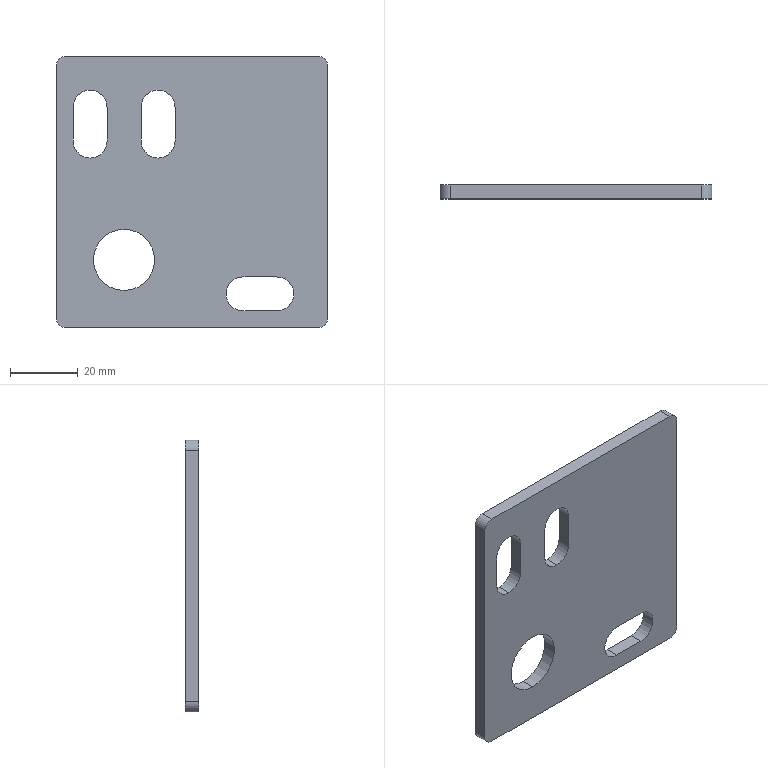Part | SolidWorks | features Extrusion 1, Fillet 1 | 1 solid | 26 faces | box 80 x 4 x 80 mm | volume 22409 mm3 | cylinder 14 | plane 12 | commonest cylinder face diameters 10 x8 6 x4 18 x2
STEP:
#1=CARTESIAN_POINT('',(-45.,4.,55.));
#2=VERTEX_POINT('',#1);
#3=CARTESIAN_POINT('',(-50.,4.,50.));
#4=VERTEX_POINT('',#3);
#5=CARTESIAN_POINT('',(-50.,4.,55.));
#6=DIRECTION('',(0.,1.,0.));
#7=DIRECTION('',(0.,0.,1.));
#8=AXIS2_PLACEMENT_3D('',#5,#6,#7);
#9=CIRCLE('',#8,5.);
#10=EDGE_CURVE('',#2,#4,#9,.T.);
#11=ORIENTED_EDGE('',*,*,#10,.T.);
#12=CARTESIAN_POINT('',(-50.,0.,50.));
#13=VERTEX_POINT('',#12);
#14=CARTESIAN_POINT('',(-50.,4.,50.));
#15=DIRECTION('',(0.,-1.,0.));
#16=VECTOR('',#15,1000.);
#17=LINE('',#14,#16);
#18=EDGE_CURVE('',#4,#13,#17,.T.);
#19=ORIENTED_EDGE('',*,*,#18,.T.);
#20=CARTESIAN_POINT('',(-45.,0.,55.));
#21=VERTEX_POINT('',#20);
#22=CARTESIAN_POINT('',(-50.,0.,55.));
#23=DIRECTION('',(0.,1.,0.));
#24=DIRECTION('',(0.,0.,1.));
#25=AXIS2_PLACEMENT_3D('',#22,#23,#24);
#26=CIRCLE('',#25,5.);
#27=EDGE_CURVE('',#21,#13,#26,.T.);
#28=ORIENTED_EDGE('',*,*,#27,.F.);
#29=CARTESIAN_POINT('',(-45.,4.,55.));
#30=DIRECTION('',(0.,-1.,0.));
#31=VECTOR('',#30,1000.);
#32=LINE('',#29,#31);
#33=EDGE_CURVE('',#2,#21,#32,.T.);
#34=ORIENTED_EDGE('',*,*,#33,.F.);
#35=EDGE_LOOP('',(#11,#19,#28,#34));
#36=FACE_OUTER_BOUND('',#35,.T.);
#37=CARTESIAN_POINT('',(-50.,4.,55.));
#38=DIRECTION('',(0.,-1.,0.));
#39=DIRECTION('',(0.,0.,-1.));
#40=AXIS2_PLACEMENT_3D('',#37,#38,#39);
#41=CYLINDRICAL_SURFACE('',#40,5.);
#42=ADVANCED_FACE('',(#36),#41,.F.);
#43=CARTESIAN_POINT('',(-65.,4.,55.));
#44=VERTEX_POINT('',#43);
#45=CARTESIAN_POINT('',(-70.,4.,50.));
#46=VERTEX_POINT('',#45);
#47=CARTESIAN_POINT('',(-70.,4.,55.));
#48=DIRECTION('',(0.,1.,0.));
#49=DIRECTION('',(0.,0.,1.));
#50=AXIS2_PLACEMENT_3D('',#47,#48,#49);
#51=CIRCLE('',#50,5.);
#52=EDGE_CURVE('',#44,#46,#51,.T.);
#53=ORIENTED_EDGE('',*,*,#52,.T.);
#54=CARTESIAN_POINT('',(-70.,0.,50.));
#55=VERTEX_POINT('',#54);
#56=CARTESIAN_POINT('',(-70.,4.,50.));
#57=DIRECTION('',(0.,-1.,0.));
#58=VECTOR('',#57,1000.);
#59=LINE('',#56,#58);
#60=EDGE_CURVE('',#46,#55,#59,.T.);
#61=ORIENTED_EDGE('',*,*,#60,.T.);
#62=CARTESIAN_POINT('',(-65.,0.,55.));
#63=VERTEX_POINT('',#62);
#64=CARTESIAN_POINT('',(-70.,0.,55.));
#65=DIRECTION('',(0.,1.,0.));
#66=DIRECTION('',(0.,0.,1.));
#67=AXIS2_PLACEMENT_3D('',#64,#65,#66);
#68=CIRCLE('',#67,5.);
#69=EDGE_CURVE('',#63,#55,#68,.T.);
#70=ORIENTED_EDGE('',*,*,#69,.F.);
#71=CARTESIAN_POINT('',(-65.,4.,55.));
#72=DIRECTION('',(0.,-1.,0.));
#73=VECTOR('',#72,1000.);
#74=LINE('',#71,#73);
#75=EDGE_CURVE('',#44,#63,#74,.T.);
#76=ORIENTED_EDGE('',*,*,#75,.F.);
#77=EDGE_LOOP('',(#53,#61,#70,#76));
#78=FACE_OUTER_BOUND('',#77,.T.);
#79=CARTESIAN_POINT('',(-70.,4.,55.));
#80=DIRECTION('',(0.,-1.,0.));
#81=DIRECTION('',(0.,0.,-1.));
#82=AXIS2_PLACEMENT_3D('',#79,#80,#81);
#83=CYLINDRICAL_SURFACE('',#82,5.);
#84=ADVANCED_FACE('',(#78),#83,.F.);
#85=CARTESIAN_POINT('',(-60.,4.,11.));
#86=VERTEX_POINT('',#85);
#87=CARTESIAN_POINT('',(-60.,4.,29.));
#88=VERTEX_POINT('',#87);
#89=CARTESIAN_POINT('',(-60.,4.,20.));
#90=DIRECTION('',(0.,1.,0.));
#91=DIRECTION('',(0.,0.,1.));
#92=AXIS2_PLACEMENT_3D('',#89,#90,#91);
#93=CIRCLE('',#92,9.);
#94=EDGE_CURVE('',#86,#88,#93,.T.);
#95=ORIENTED_EDGE('',*,*,#94,.T.);
#96=CARTESIAN_POINT('',(-60.,0.,29.));
#97=VERTEX_POINT('',#96);
#98=CARTESIAN_POINT('',(-60.,4.,29.));
#99=DIRECTION('',(0.,-1.,0.));
#100=VECTOR('',#99,1000.);
#101=LINE('',#98,#100);
#102=EDGE_CURVE('',#88,#97,#101,.T.);
#103=ORIENTED_EDGE('',*,*,#102,.T.);
#104=CARTESIAN_POINT('',(-60.,0.,11.));
#105=VERTEX_POINT('',#104);
#106=CARTESIAN_POINT('',(-60.,0.,20.));
#107=DIRECTION('',(0.,1.,0.));
#108=DIRECTION('',(0.,0.,1.));
#109=AXIS2_PLACEMENT_3D('',#106,#107,#108);
#110=CIRCLE('',#109,9.);
#111=EDGE_CURVE('',#105,#97,#110,.T.);
#112=ORIENTED_EDGE('',*,*,#111,.F.);
#113=CARTESIAN_POINT('',(-60.,4.,11.));
#114=DIRECTION('',(0.,-1.,0.));
#115=VECTOR('',#114,1000.);
#116=LINE('',#113,#115);
#117=EDGE_CURVE('',#86,#105,#116,.T.);
#118=ORIENTED_EDGE('',*,*,#117,.F.);
#119=EDGE_LOOP('',(#95,#103,#112,#118));
#120=FACE_OUTER_BOUND('',#119,.T.);
#121=CARTESIAN_POINT('',(-60.,4.,20.));
#122=DIRECTION('',(0.,-1.,0.));
#123=DIRECTION('',(0.,0.,-1.));
#124=AXIS2_PLACEMENT_3D('',#121,#122,#123);
#125=CYLINDRICAL_SURFACE('',#124,9.);
#126=ADVANCED_FACE('',(#120),#125,.F.);
#127=CARTESIAN_POINT('',(-77.,4.,80.));
#128=VERTEX_POINT('',#127);
#129=CARTESIAN_POINT('',(-3.,4.,80.));
#130=VERTEX_POINT('',#129);
#131=CARTESIAN_POINT('',(-80.,4.,80.));
#132=DIRECTION('',(1.,0.,0.));
#133=VECTOR('',#132,1000.);
#134=LINE('',#131,#133);
#135=EDGE_CURVE('',#128,#130,#134,.T.);
#136=ORIENTED_EDGE('',*,*,#135,.T.);
#137=CARTESIAN_POINT('',(0.,4.,77.));
#138=VERTEX_POINT('',#137);
#139=CARTESIAN_POINT('',(-3.,4.,77.));
#140=DIRECTION('',(0.,1.,0.));
#141=DIRECTION('',(0.,0.,1.));
#142=AXIS2_PLACEMENT_3D('',#139,#140,#141);
#143=CIRCLE('',#142,3.);
#144=EDGE_CURVE('',#130,#138,#143,.T.);
#145=ORIENTED_EDGE('',*,*,#144,.T.);
#146=CARTESIAN_POINT('',(0.,4.,3.));
#147=VERTEX_POINT('',#146);
#148=CARTESIAN_POINT('',(0.,4.,80.));
#149=DIRECTION('',(0.,0.,-1.));
#150=VECTOR('',#149,1000.);
#151=LINE('',#148,#150);
#152=EDGE_CURVE('',#138,#147,#151,.T.);
#153=ORIENTED_EDGE('',*,*,#152,.T.);
#154=CARTESIAN_POINT('',(-3.,4.,0.));
#155=VERTEX_POINT('',#154);
#156=CARTESIAN_POINT('',(-3.,4.,3.));
#157=DIRECTION('',(0.,1.,0.));
#158=DIRECTION('',(0.,0.,1.));
#159=AXIS2_PLACEMENT_3D('',#156,#157,#158);
#160=CIRCLE('',#159,3.);
#161=EDGE_CURVE('',#147,#155,#160,.T.);
#162=ORIENTED_EDGE('',*,*,#161,.T.);
#163=CARTESIAN_POINT('',(-77.,4.,0.));
#164=VERTEX_POINT('',#163);
#165=CARTESIAN_POINT('',(0.,4.,0.));
#166=DIRECTION('',(-1.,0.,0.));
#167=VECTOR('',#166,1000.);
#168=LINE('',#165,#167);
#169=EDGE_CURVE('',#155,#164,#168,.T.);
#170=ORIENTED_EDGE('',*,*,#169,.T.);
#171=CARTESIAN_POINT('',(-80.,4.,3.));
#172=VERTEX_POINT('',#171);
#173=CARTESIAN_POINT('',(-77.,4.,3.));
#174=DIRECTION('',(0.,1.,0.));
#175=DIRECTION('',(0.,0.,1.));
#176=AXIS2_PLACEMENT_3D('',#173,#174,#175);
#177=CIRCLE('',#176,3.);
#178=EDGE_CURVE('',#164,#172,#177,.T.);
#179=ORIENTED_EDGE('',*,*,#178,.T.);
#180=CARTESIAN_POINT('',(-80.,4.,77.));
#181=VERTEX_POINT('',#180);
#182=CARTESIAN_POINT('',(-80.,4.,0.));
#183=DIRECTION('',(0.,0.,1.));
#184=VECTOR('',#183,1000.);
#185=LINE('',#182,#184);
#186=EDGE_CURVE('',#172,#181,#185,.T.);
#187=ORIENTED_EDGE('',*,*,#186,.T.);
#188=CARTESIAN_POINT('',(-77.,4.,77.));
#189=DIRECTION('',(0.,1.,0.));
#190=DIRECTION('',(0.,0.,1.));
#191=AXIS2_PLACEMENT_3D('',#188,#189,#190);
#192=CIRCLE('',#191,3.);
#193=EDGE_CURVE('',#181,#128,#192,.T.);
#194=ORIENTED_EDGE('',*,*,#193,.T.);
#195=EDGE_LOOP('',(#136,#145,#153,#162,#170,#179,#187,#194));
#196=FACE_OUTER_BOUND('',#195,.T.);
#197=ORIENTED_EDGE('',*,*,#94,.F.);
#198=CARTESIAN_POINT('',(-60.,4.,20.));
#199=DIRECTION('',(0.,1.,0.));
#200=DIRECTION('',(0.,0.,1.));
#201=AXIS2_PLACEMENT_3D('',#198,#199,#200);
#202=CIRCLE('',#201,9.);
#203=EDGE_CURVE('',#88,#86,#202,.T.);
#204=ORIENTED_EDGE('',*,*,#203,.F.);
#205=EDGE_LOOP('',(#197,#204));
#206=FACE_BOUND('',#205,.T.);
#207=CARTESIAN_POINT('',(-25.,4.,15.));
#208=VERTEX_POINT('',#207);
#209=CARTESIAN_POINT('',(-15.,4.,15.));
#210=VERTEX_POINT('',#209);
#211=CARTESIAN_POINT('',(-25.,4.,15.));
#212=DIRECTION('',(1.,0.,0.));
#213=VECTOR('',#212,1000.);
#214=LINE('',#211,#213);
#215=EDGE_CURVE('',#208,#210,#214,.T.);
#216=ORIENTED_EDGE('',*,*,#215,.F.);
#217=CARTESIAN_POINT('',(-25.,4.,5.));
#218=VERTEX_POINT('',#217);
#219=CARTESIAN_POINT('',(-25.,4.,10.));
#220=DIRECTION('',(0.,1.,0.));
#221=DIRECTION('',(0.,0.,1.));
#222=AXIS2_PLACEMENT_3D('',#219,#220,#221);
#223=CIRCLE('',#222,5.);
#224=EDGE_CURVE('',#218,#208,#223,.T.);
#225=ORIENTED_EDGE('',*,*,#224,.F.);
#226=CARTESIAN_POINT('',(-15.,4.,5.));
#227=VERTEX_POINT('',#226);
#228=CARTESIAN_POINT('',(-25.,4.,5.));
#229=DIRECTION('',(-1.,0.,0.));
#230=VECTOR('',#229,1000.);
#231=LINE('',#228,#230);
#232=EDGE_CURVE('',#227,#218,#231,.T.);
#233=ORIENTED_EDGE('',*,*,#232,.F.);
#234=CARTESIAN_POINT('',(-15.,4.,10.));
#235=DIRECTION('',(0.,1.,0.));
#236=DIRECTION('',(0.,0.,1.));
#237=AXIS2_PLACEMENT_3D('',#234,#235,#236);
#238=CIRCLE('',#237,5.);
#239=EDGE_CURVE('',#210,#227,#238,.T.);
#240=ORIENTED_EDGE('',*,*,#239,.F.);
#241=EDGE_LOOP('',(#216,#225,#233,#240));
#242=FACE_BOUND('',#241,.T.);
#243=CARTESIAN_POINT('',(-75.,4.,55.));
#244=VERTEX_POINT('',#243);
#245=CARTESIAN_POINT('',(-75.,4.,65.));
#246=VERTEX_POINT('',#245);
#247=CARTESIAN_POINT('',(-75.,4.,55.));
#248=DIRECTION('',(0.,0.,1.));
#249=VECTOR('',#248,1000.);
#250=LINE('',#247,#249);
#251=EDGE_CURVE('',#244,#246,#250,.T.);
#252=ORIENTED_EDGE('',*,*,#251,.F.);
#253=CARTESIAN_POINT('',(-70.,4.,55.));
#254=DIRECTION('',(0.,1.,0.));
#255=DIRECTION('',(0.,0.,1.));
#256=AXIS2_PLACEMENT_3D('',#253,#254,#255);
#257=CIRCLE('',#256,5.);
#258=EDGE_CURVE('',#46,#244,#257,.T.);
#259=ORIENTED_EDGE('',*,*,#258,.F.);
#260=ORIENTED_EDGE('',*,*,#52,.F.);
#261=CARTESIAN_POINT('',(-65.,4.,65.));
#262=VERTEX_POINT('',#261);
#263=CARTESIAN_POINT('',(-65.,4.,55.));
#264=DIRECTION('',(0.,0.,-1.));
#265=VECTOR('',#264,1000.);
#266=LINE('',#263,#265);
#267=EDGE_CURVE('',#262,#44,#266,.T.);
#268=ORIENTED_EDGE('',*,*,#267,.F.);
#269=CARTESIAN_POINT('',(-70.,4.,65.));
#270=DIRECTION('',(0.,1.,0.));
#271=DIRECTION('',(0.,0.,1.));
#272=AXIS2_PLACEMENT_3D('',#269,#270,#271);
#273=CIRCLE('',#272,5.);
#274=EDGE_CURVE('',#246,#262,#273,.T.);
#275=ORIENTED_EDGE('',*,*,#274,.F.);
#276=EDGE_LOOP('',(#252,#259,#260,#268,#275));
#277=FACE_BOUND('',#276,.T.);
#278=CARTESIAN_POINT('',(-55.,4.,55.));
#279=VERTEX_POINT('',#278);
#280=CARTESIAN_POINT('',(-55.,4.,65.));
#281=VERTEX_POINT('',#280);
#282=CARTESIAN_POINT('',(-55.,4.,55.));
#283=DIRECTION('',(0.,0.,1.));
#284=VECTOR('',#283,1000.);
#285=LINE('',#282,#284);
#286=EDGE_CURVE('',#279,#281,#285,.T.);
#287=ORIENTED_EDGE('',*,*,#286,.F.);
#288=CARTESIAN_POINT('',(-50.,4.,55.));
#289=DIRECTION('',(0.,1.,0.));
#290=DIRECTION('',(0.,0.,1.));
#291=AXIS2_PLACEMENT_3D('',#288,#289,#290);
#292=CIRCLE('',#291,5.);
#293=EDGE_CURVE('',#4,#279,#292,.T.);
#294=ORIENTED_EDGE('',*,*,#293,.F.);
#295=ORIENTED_EDGE('',*,*,#10,.F.);
#296=CARTESIAN_POINT('',(-45.,4.,65.));
#297=VERTEX_POINT('',#296);
#298=CARTESIAN_POINT('',(-45.,4.,55.));
#299=DIRECTION('',(0.,0.,-1.));
#300=VECTOR('',#299,1000.);
#301=LINE('',#298,#300);
#302=EDGE_CURVE('',#297,#2,#301,.T.);
#303=ORIENTED_EDGE('',*,*,#302,.F.);
#304=CARTESIAN_POINT('',(-50.,4.,65.));
#305=DIRECTION('',(0.,1.,0.));
#306=DIRECTION('',(0.,0.,1.));
#307=AXIS2_PLACEMENT_3D('',#304,#305,#306);
#308=CIRCLE('',#307,5.);
#309=EDGE_CURVE('',#281,#297,#308,.T.);
#310=ORIENTED_EDGE('',*,*,#309,.F.);
#311=EDGE_LOOP('',(#287,#294,#295,#303,#310));
#312=FACE_BOUND('',#311,.T.);
#313=CARTESIAN_POINT('',(0.,4.,0.));
#314=DIRECTION('',(0.,1.,0.));
#315=DIRECTION('',(0.,0.,1.));
#316=AXIS2_PLACEMENT_3D('',#313,#314,#315);
#317=PLANE('',#316);
#318=ADVANCED_FACE('',(#196,#206,#242,#277,#312),#317,.T.);
#319=ORIENTED_EDGE('',*,*,#69,.T.);
#320=CARTESIAN_POINT('',(-75.,0.,55.));
#321=VERTEX_POINT('',#320);
#322=CARTESIAN_POINT('',(-70.,0.,55.));
#323=DIRECTION('',(0.,1.,0.));
#324=DIRECTION('',(0.,0.,1.));
#325=AXIS2_PLACEMENT_3D('',#322,#323,#324);
#326=CIRCLE('',#325,5.);
#327=EDGE_CURVE('',#55,#321,#326,.T.);
#328=ORIENTED_EDGE('',*,*,#327,.T.);
#329=CARTESIAN_POINT('',(-75.,0.,65.));
#330=VERTEX_POINT('',#329);
#331=CARTESIAN_POINT('',(-75.,0.,55.));
#332=DIRECTION('',(0.,0.,1.));
#333=VECTOR('',#332,1000.);
#334=LINE('',#331,#333);
#335=EDGE_CURVE('',#321,#330,#334,.T.);
#336=ORIENTED_EDGE('',*,*,#335,.T.);
#337=CARTESIAN_POINT('',(-65.,0.,65.));
#338=VERTEX_POINT('',#337);
#339=CARTESIAN_POINT('',(-70.,0.,65.));
#340=DIRECTION('',(0.,1.,0.));
#341=DIRECTION('',(0.,0.,1.));
#342=AXIS2_PLACEMENT_3D('',#339,#340,#341);
#343=CIRCLE('',#342,5.);
#344=EDGE_CURVE('',#330,#338,#343,.T.);
#345=ORIENTED_EDGE('',*,*,#344,.T.);
#346=CARTESIAN_POINT('',(-65.,0.,55.));
#347=DIRECTION('',(0.,0.,-1.));
#348=VECTOR('',#347,1000.);
#349=LINE('',#346,#348);
#350=EDGE_CURVE('',#338,#63,#349,.T.);
#351=ORIENTED_EDGE('',*,*,#350,.T.);
#352=EDGE_LOOP('',(#319,#328,#336,#345,#351));
#353=FACE_BOUND('',#352,.T.);
#354=ORIENTED_EDGE('',*,*,#111,.T.);
#355=CARTESIAN_POINT('',(-60.,0.,20.));
#356=DIRECTION('',(0.,1.,0.));
#357=DIRECTION('',(0.,0.,1.));
#358=AXIS2_PLACEMENT_3D('',#355,#356,#357);
#359=CIRCLE('',#358,9.);
#360=EDGE_CURVE('',#97,#105,#359,.T.);
#361=ORIENTED_EDGE('',*,*,#360,.T.);
#362=EDGE_LOOP('',(#354,#361));
#363=FACE_BOUND('',#362,.T.);
#364=CARTESIAN_POINT('',(0.,0.,77.));
#365=VERTEX_POINT('',#364);
#366=CARTESIAN_POINT('',(0.,0.,3.));
#367=VERTEX_POINT('',#366);
#368=CARTESIAN_POINT('',(0.,0.,80.));
#369=DIRECTION('',(0.,0.,-1.));
#370=VECTOR('',#369,1000.);
#371=LINE('',#368,#370);
#372=EDGE_CURVE('',#365,#367,#371,.T.);
#373=ORIENTED_EDGE('',*,*,#372,.F.);
#374=CARTESIAN_POINT('',(-3.,0.,80.));
#375=VERTEX_POINT('',#374);
#376=CARTESIAN_POINT('',(-3.,0.,77.));
#377=DIRECTION('',(0.,-1.,0.));
#378=DIRECTION('',(0.,0.,1.));
#379=AXIS2_PLACEMENT_3D('',#376,#377,#378);
#380=CIRCLE('',#379,3.);
#381=EDGE_CURVE('',#365,#375,#380,.T.);
#382=ORIENTED_EDGE('',*,*,#381,.T.);
#383=CARTESIAN_POINT('',(-77.,0.,80.));
#384=VERTEX_POINT('',#383);
#385=CARTESIAN_POINT('',(-80.,0.,80.));
#386=DIRECTION('',(1.,0.,0.));
#387=VECTOR('',#386,1000.);
#388=LINE('',#385,#387);
#389=EDGE_CURVE('',#384,#375,#388,.T.);
#390=ORIENTED_EDGE('',*,*,#389,.F.);
#391=CARTESIAN_POINT('',(-80.,0.,77.));
#392=VERTEX_POINT('',#391);
#393=CARTESIAN_POINT('',(-77.,0.,77.));
#394=DIRECTION('',(0.,-1.,0.));
#395=DIRECTION('',(0.,0.,1.));
#396=AXIS2_PLACEMENT_3D('',#393,#394,#395);
#397=CIRCLE('',#396,3.);
#398=EDGE_CURVE('',#384,#392,#397,.T.);
#399=ORIENTED_EDGE('',*,*,#398,.T.);
#400=CARTESIAN_POINT('',(-80.,0.,3.));
#401=VERTEX_POINT('',#400);
#402=CARTESIAN_POINT('',(-80.,0.,0.));
#403=DIRECTION('',(0.,0.,1.));
#404=VECTOR('',#403,1000.);
#405=LINE('',#402,#404);
#406=EDGE_CURVE('',#401,#392,#405,.T.);
#407=ORIENTED_EDGE('',*,*,#406,.F.);
#408=CARTESIAN_POINT('',(-77.,0.,0.));
#409=VERTEX_POINT('',#408);
#410=CARTESIAN_POINT('',(-77.,0.,3.));
#411=DIRECTION('',(0.,-1.,0.));
#412=DIRECTION('',(0.,0.,1.));
#413=AXIS2_PLACEMENT_3D('',#410,#411,#412);
#414=CIRCLE('',#413,3.);
#415=EDGE_CURVE('',#401,#409,#414,.T.);
#416=ORIENTED_EDGE('',*,*,#415,.T.);
#417=CARTESIAN_POINT('',(-3.,0.,0.));
#418=VERTEX_POINT('',#417);
#419=CARTESIAN_POINT('',(0.,0.,0.));
#420=DIRECTION('',(-1.,0.,0.));
#421=VECTOR('',#420,1000.);
#422=LINE('',#419,#421);
#423=EDGE_CURVE('',#418,#409,#422,.T.);
#424=ORIENTED_EDGE('',*,*,#423,.F.);
#425=CARTESIAN_POINT('',(-3.,0.,3.));
#426=DIRECTION('',(0.,-1.,0.));
#427=DIRECTION('',(0.,0.,1.));
#428=AXIS2_PLACEMENT_3D('',#425,#426,#427);
#429=CIRCLE('',#428,3.);
#430=EDGE_CURVE('',#418,#367,#429,.T.);
#431=ORIENTED_EDGE('',*,*,#430,.T.);
#432=EDGE_LOOP('',(#373,#382,#390,#399,#407,#416,#424,#431));
#433=FACE_OUTER_BOUND('',#432,.T.);
#434=CARTESIAN_POINT('',(-25.,0.,5.));
#435=VERTEX_POINT('',#434);
#436=CARTESIAN_POINT('',(-25.,0.,15.));
#437=VERTEX_POINT('',#436);
#438=CARTESIAN_POINT('',(-25.,0.,10.));
#439=DIRECTION('',(0.,1.,0.));
#440=DIRECTION('',(0.,0.,1.));
#441=AXIS2_PLACEMENT_3D('',#438,#439,#440);
#442=CIRCLE('',#441,5.);
#443=EDGE_CURVE('',#435,#437,#442,.T.);
#444=ORIENTED_EDGE('',*,*,#443,.T.);
#445=CARTESIAN_POINT('',(-15.,0.,15.));
#446=VERTEX_POINT('',#445);
#447=CARTESIAN_POINT('',(-25.,0.,15.));
#448=DIRECTION('',(1.,0.,0.));
#449=VECTOR('',#448,1000.);
#450=LINE('',#447,#449);
#451=EDGE_CURVE('',#437,#446,#450,.T.);
#452=ORIENTED_EDGE('',*,*,#451,.T.);
#453=CARTESIAN_POINT('',(-15.,0.,5.));
#454=VERTEX_POINT('',#453);
#455=CARTESIAN_POINT('',(-15.,0.,10.));
#456=DIRECTION('',(0.,1.,0.));
#457=DIRECTION('',(0.,0.,1.));
#458=AXIS2_PLACEMENT_3D('',#455,#456,#457);
#459=CIRCLE('',#458,5.);
#460=EDGE_CURVE('',#446,#454,#459,.T.);
#461=ORIENTED_EDGE('',*,*,#460,.T.);
#462=CARTESIAN_POINT('',(-25.,0.,5.));
#463=DIRECTION('',(-1.,0.,0.));
#464=VECTOR('',#463,1000.);
#465=LINE('',#462,#464);
#466=EDGE_CURVE('',#454,#435,#465,.T.);
#467=ORIENTED_EDGE('',*,*,#466,.T.);
#468=EDGE_LOOP('',(#444,#452,#461,#467));
#469=FACE_BOUND('',#468,.T.);
#470=ORIENTED_EDGE('',*,*,#27,.T.);
#471=CARTESIAN_POINT('',(-55.,0.,55.));
#472=VERTEX_POINT('',#471);
#473=CARTESIAN_POINT('',(-50.,0.,55.));
#474=DIRECTION('',(0.,1.,0.));
#475=DIRECTION('',(0.,0.,1.));
#476=AXIS2_PLACEMENT_3D('',#473,#474,#475);
#477=CIRCLE('',#476,5.);
#478=EDGE_CURVE('',#13,#472,#477,.T.);
#479=ORIENTED_EDGE('',*,*,#478,.T.);
#480=CARTESIAN_POINT('',(-55.,0.,65.));
#481=VERTEX_POINT('',#480);
#482=CARTESIAN_POINT('',(-55.,0.,55.));
#483=DIRECTION('',(0.,0.,1.));
#484=VECTOR('',#483,1000.);
#485=LINE('',#482,#484);
#486=EDGE_CURVE('',#472,#481,#485,.T.);
#487=ORIENTED_EDGE('',*,*,#486,.T.);
#488=CARTESIAN_POINT('',(-45.,0.,65.));
#489=VERTEX_POINT('',#488);
#490=CARTESIAN_POINT('',(-50.,0.,65.));
#491=DIRECTION('',(0.,1.,0.));
#492=DIRECTION('',(0.,0.,1.));
#493=AXIS2_PLACEMENT_3D('',#490,#491,#492);
#494=CIRCLE('',#493,5.);
#495=EDGE_CURVE('',#481,#489,#494,.T.);
#496=ORIENTED_EDGE('',*,*,#495,.T.);
#497=CARTESIAN_POINT('',(-45.,0.,55.));
#498=DIRECTION('',(0.,0.,-1.));
#499=VECTOR('',#498,1000.);
#500=LINE('',#497,#499);
#501=EDGE_CURVE('',#489,#21,#500,.T.);
#502=ORIENTED_EDGE('',*,*,#501,.T.);
#503=EDGE_LOOP('',(#470,#479,#487,#496,#502));
#504=FACE_BOUND('',#503,.T.);
#505=CARTESIAN_POINT('',(0.,0.,0.));
#506=DIRECTION('',(0.,1.,0.));
#507=DIRECTION('',(0.,0.,1.));
#508=AXIS2_PLACEMENT_3D('',#505,#506,#507);
#509=PLANE('',#508);
#510=ADVANCED_FACE('',(#353,#363,#433,#469,#504),#509,.F.);
#511=ORIENTED_EDGE('',*,*,#152,.F.);
#512=CARTESIAN_POINT('',(0.,4.,77.));
#513=DIRECTION('',(0.,-1.,0.));
#514=VECTOR('',#513,1000.);
#515=LINE('',#512,#514);
#516=EDGE_CURVE('',#138,#365,#515,.T.);
#517=ORIENTED_EDGE('',*,*,#516,.T.);
#518=ORIENTED_EDGE('',*,*,#372,.T.);
#519=CARTESIAN_POINT('',(0.,4.,3.));
#520=DIRECTION('',(0.,1.,0.));
#521=VECTOR('',#520,1000.);
#522=LINE('',#519,#521);
#523=EDGE_CURVE('',#367,#147,#522,.T.);
#524=ORIENTED_EDGE('',*,*,#523,.T.);
#525=EDGE_LOOP('',(#511,#517,#518,#524));
#526=FACE_OUTER_BOUND('',#525,.T.);
#527=CARTESIAN_POINT('',(0.,4.,80.));
#528=DIRECTION('',(-1.,0.,0.));
#529=DIRECTION('',(0.,0.,1.));
#530=AXIS2_PLACEMENT_3D('',#527,#528,#529);
#531=PLANE('',#530);
#532=ADVANCED_FACE('',(#526),#531,.F.);
#533=ORIENTED_EDGE('',*,*,#169,.F.);
#534=CARTESIAN_POINT('',(-3.,4.,0.));
#535=DIRECTION('',(0.,-1.,0.));
#536=VECTOR('',#535,1000.);
#537=LINE('',#534,#536);
#538=EDGE_CURVE('',#155,#418,#537,.T.);
#539=ORIENTED_EDGE('',*,*,#538,.T.);
#540=ORIENTED_EDGE('',*,*,#423,.T.);
#541=CARTESIAN_POINT('',(-77.,4.,0.));
#542=DIRECTION('',(0.,1.,0.));
#543=VECTOR('',#542,1000.);
#544=LINE('',#541,#543);
#545=EDGE_CURVE('',#409,#164,#544,.T.);
#546=ORIENTED_EDGE('',*,*,#545,.T.);
#547=EDGE_LOOP('',(#533,#539,#540,#546));
#548=FACE_OUTER_BOUND('',#547,.T.);
#549=CARTESIAN_POINT('',(0.,4.,0.));
#550=DIRECTION('',(0.,0.,1.));
#551=DIRECTION('',(1.,0.,0.));
#552=AXIS2_PLACEMENT_3D('',#549,#550,#551);
#553=PLANE('',#552);
#554=ADVANCED_FACE('',(#548),#553,.F.);
#555=ORIENTED_EDGE('',*,*,#406,.T.);
#556=CARTESIAN_POINT('',(-80.,4.,77.));
#557=DIRECTION('',(0.,1.,0.));
#558=VECTOR('',#557,1000.);
#559=LINE('',#556,#558);
#560=EDGE_CURVE('',#392,#181,#559,.T.);
#561=ORIENTED_EDGE('',*,*,#560,.T.);
#562=ORIENTED_EDGE('',*,*,#186,.F.);
#563=CARTESIAN_POINT('',(-80.,4.,3.));
#564=DIRECTION('',(0.,-1.,0.));
#565=VECTOR('',#564,1000.);
#566=LINE('',#563,#565);
#567=EDGE_CURVE('',#172,#401,#566,.T.);
#568=ORIENTED_EDGE('',*,*,#567,.T.);
#569=EDGE_LOOP('',(#555,#561,#562,#568));
#570=FACE_OUTER_BOUND('',#569,.T.);
#571=CARTESIAN_POINT('',(-80.,4.,0.));
#572=DIRECTION('',(1.,0.,0.));
#573=DIRECTION('',(0.,0.,-1.));
#574=AXIS2_PLACEMENT_3D('',#571,#572,#573);
#575=PLANE('',#574);
#576=ADVANCED_FACE('',(#570),#575,.F.);
#577=ORIENTED_EDGE('',*,*,#389,.T.);
#578=CARTESIAN_POINT('',(-3.,4.,80.));
#579=DIRECTION('',(0.,1.,0.));
#580=VECTOR('',#579,1000.);
#581=LINE('',#578,#580);
#582=EDGE_CURVE('',#375,#130,#581,.T.);
#583=ORIENTED_EDGE('',*,*,#582,.T.);
#584=ORIENTED_EDGE('',*,*,#135,.F.);
#585=CARTESIAN_POINT('',(-77.,4.,80.));
#586=DIRECTION('',(0.,-1.,0.));
#587=VECTOR('',#586,1000.);
#588=LINE('',#585,#587);
#589=EDGE_CURVE('',#128,#384,#588,.T.);
#590=ORIENTED_EDGE('',*,*,#589,.T.);
#591=EDGE_LOOP('',(#577,#583,#584,#590));
#592=FACE_OUTER_BOUND('',#591,.T.);
#593=CARTESIAN_POINT('',(-80.,4.,80.));
#594=DIRECTION('',(0.,0.,-1.));
#595=DIRECTION('',(-1.,0.,0.));
#596=AXIS2_PLACEMENT_3D('',#593,#594,#595);
#597=PLANE('',#596);
#598=ADVANCED_FACE('',(#592),#597,.F.);
#599=ORIENTED_EDGE('',*,*,#102,.F.);
#600=ORIENTED_EDGE('',*,*,#203,.T.);
#601=ORIENTED_EDGE('',*,*,#117,.T.);
#602=ORIENTED_EDGE('',*,*,#360,.F.);
#603=EDGE_LOOP('',(#599,#600,#601,#602));
#604=FACE_OUTER_BOUND('',#603,.T.);
#605=CARTESIAN_POINT('',(-60.,4.,20.));
#606=DIRECTION('',(0.,-1.,0.));
#607=DIRECTION('',(0.,0.,-1.));
#608=AXIS2_PLACEMENT_3D('',#605,#606,#607);
#609=CYLINDRICAL_SURFACE('',#608,9.);
#610=ADVANCED_FACE('',(#604),#609,.F.);
#611=ORIENTED_EDGE('',*,*,#443,.F.);
#612=CARTESIAN_POINT('',(-25.,4.,5.));
#613=DIRECTION('',(0.,-1.,0.));
#614=VECTOR('',#613,1000.);
#615=LINE('',#612,#614);
#616=EDGE_CURVE('',#218,#435,#615,.T.);
#617=ORIENTED_EDGE('',*,*,#616,.F.);
#618=ORIENTED_EDGE('',*,*,#224,.T.);
#619=CARTESIAN_POINT('',(-25.,4.,15.));
#620=DIRECTION('',(0.,-1.,0.));
#621=VECTOR('',#620,1000.);
#622=LINE('',#619,#621);
#623=EDGE_CURVE('',#208,#437,#622,.T.);
#624=ORIENTED_EDGE('',*,*,#623,.T.);
#625=EDGE_LOOP('',(#611,#617,#618,#624));
#626=FACE_OUTER_BOUND('',#625,.T.);
#627=CARTESIAN_POINT('',(-25.,4.,10.));
#628=DIRECTION('',(0.,-1.,0.));
#629=DIRECTION('',(0.,0.,-1.));
#630=AXIS2_PLACEMENT_3D('',#627,#628,#629);
#631=CYLINDRICAL_SURFACE('',#630,5.);
#632=ADVANCED_FACE('',(#626),#631,.F.);
#633=ORIENTED_EDGE('',*,*,#451,.F.);
#634=ORIENTED_EDGE('',*,*,#623,.F.);
#635=ORIENTED_EDGE('',*,*,#215,.T.);
#636=CARTESIAN_POINT('',(-15.,4.,15.));
#637=DIRECTION('',(0.,-1.,0.));
#638=VECTOR('',#637,1000.);
#639=LINE('',#636,#638);
#640=EDGE_CURVE('',#210,#446,#639,.T.);
#641=ORIENTED_EDGE('',*,*,#640,.T.);
#642=EDGE_LOOP('',(#633,#634,#635,#641));
#643=FACE_OUTER_BOUND('',#642,.T.);
#644=CARTESIAN_POINT('',(-25.,4.,15.));
#645=DIRECTION('',(0.,0.,-1.));
#646=DIRECTION('',(-1.,0.,0.));
#647=AXIS2_PLACEMENT_3D('',#644,#645,#646);
#648=PLANE('',#647);
#649=ADVANCED_FACE('',(#643),#648,.T.);
#650=ORIENTED_EDGE('',*,*,#460,.F.);
#651=ORIENTED_EDGE('',*,*,#640,.F.);
#652=ORIENTED_EDGE('',*,*,#239,.T.);
#653=CARTESIAN_POINT('',(-15.,4.,5.));
#654=DIRECTION('',(0.,-1.,0.));
#655=VECTOR('',#654,1000.);
#656=LINE('',#653,#655);
#657=EDGE_CURVE('',#227,#454,#656,.T.);
#658=ORIENTED_EDGE('',*,*,#657,.T.);
#659=EDGE_LOOP('',(#650,#651,#652,#658));
#660=FACE_OUTER_BOUND('',#659,.T.);
#661=CARTESIAN_POINT('',(-15.,4.,10.));
#662=DIRECTION('',(0.,-1.,0.));
#663=DIRECTION('',(0.,0.,-1.));
#664=AXIS2_PLACEMENT_3D('',#661,#662,#663);
#665=CYLINDRICAL_SURFACE('',#664,5.);
#666=ADVANCED_FACE('',(#660),#665,.F.);
#667=ORIENTED_EDGE('',*,*,#466,.F.);
#668=ORIENTED_EDGE('',*,*,#657,.F.);
#669=ORIENTED_EDGE('',*,*,#232,.T.);
#670=ORIENTED_EDGE('',*,*,#616,.T.);
#671=EDGE_LOOP('',(#667,#668,#669,#670));
#672=FACE_OUTER_BOUND('',#671,.T.);
#673=CARTESIAN_POINT('',(-25.,4.,5.));
#674=DIRECTION('',(0.,0.,1.));
#675=DIRECTION('',(1.,0.,0.));
#676=AXIS2_PLACEMENT_3D('',#673,#674,#675);
#677=PLANE('',#676);
#678=ADVANCED_FACE('',(#672),#677,.T.);
#679=ORIENTED_EDGE('',*,*,#60,.F.);
#680=ORIENTED_EDGE('',*,*,#258,.T.);
#681=CARTESIAN_POINT('',(-75.,4.,55.));
#682=DIRECTION('',(0.,-1.,0.));
#683=VECTOR('',#682,1000.);
#684=LINE('',#681,#683);
#685=EDGE_CURVE('',#244,#321,#684,.T.);
#686=ORIENTED_EDGE('',*,*,#685,.T.);
#687=ORIENTED_EDGE('',*,*,#327,.F.);
#688=EDGE_LOOP('',(#679,#680,#686,#687));
#689=FACE_OUTER_BOUND('',#688,.T.);
#690=CARTESIAN_POINT('',(-70.,4.,55.));
#691=DIRECTION('',(0.,-1.,0.));
#692=DIRECTION('',(0.,0.,-1.));
#693=AXIS2_PLACEMENT_3D('',#690,#691,#692);
#694=CYLINDRICAL_SURFACE('',#693,5.);
#695=ADVANCED_FACE('',(#689),#694,.F.);
#696=ORIENTED_EDGE('',*,*,#335,.F.);
#697=ORIENTED_EDGE('',*,*,#685,.F.);
#698=ORIENTED_EDGE('',*,*,#251,.T.);
#699=CARTESIAN_POINT('',(-75.,4.,65.));
#700=DIRECTION('',(0.,-1.,0.));
#701=VECTOR('',#700,1000.);
#702=LINE('',#699,#701);
#703=EDGE_CURVE('',#246,#330,#702,.T.);
#704=ORIENTED_EDGE('',*,*,#703,.T.);
#705=EDGE_LOOP('',(#696,#697,#698,#704));
#706=FACE_OUTER_BOUND('',#705,.T.);
#707=CARTESIAN_POINT('',(-75.,4.,55.));
#708=DIRECTION('',(1.,0.,0.));
#709=DIRECTION('',(0.,0.,-1.));
#710=AXIS2_PLACEMENT_3D('',#707,#708,#709);
#711=PLANE('',#710);
#712=ADVANCED_FACE('',(#706),#711,.T.);
#713=ORIENTED_EDGE('',*,*,#344,.F.);
#714=ORIENTED_EDGE('',*,*,#703,.F.);
#715=ORIENTED_EDGE('',*,*,#274,.T.);
#716=CARTESIAN_POINT('',(-65.,4.,65.));
#717=DIRECTION('',(0.,-1.,0.));
#718=VECTOR('',#717,1000.);
#719=LINE('',#716,#718);
#720=EDGE_CURVE('',#262,#338,#719,.T.);
#721=ORIENTED_EDGE('',*,*,#720,.T.);
#722=EDGE_LOOP('',(#713,#714,#715,#721));
#723=FACE_OUTER_BOUND('',#722,.T.);
#724=CARTESIAN_POINT('',(-70.,4.,65.));
#725=DIRECTION('',(0.,-1.,0.));
#726=DIRECTION('',(0.,0.,-1.));
#727=AXIS2_PLACEMENT_3D('',#724,#725,#726);
#728=CYLINDRICAL_SURFACE('',#727,5.);
#729=ADVANCED_FACE('',(#723),#728,.F.);
#730=ORIENTED_EDGE('',*,*,#350,.F.);
#731=ORIENTED_EDGE('',*,*,#720,.F.);
#732=ORIENTED_EDGE('',*,*,#267,.T.);
#733=ORIENTED_EDGE('',*,*,#75,.T.);
#734=EDGE_LOOP('',(#730,#731,#732,#733));
#735=FACE_OUTER_BOUND('',#734,.T.);
#736=CARTESIAN_POINT('',(-65.,4.,55.));
#737=DIRECTION('',(-1.,0.,0.));
#738=DIRECTION('',(0.,0.,1.));
#739=AXIS2_PLACEMENT_3D('',#736,#737,#738);
#740=PLANE('',#739);
#741=ADVANCED_FACE('',(#735),#740,.T.);
#742=ORIENTED_EDGE('',*,*,#18,.F.);
#743=ORIENTED_EDGE('',*,*,#293,.T.);
#744=CARTESIAN_POINT('',(-55.,4.,55.));
#745=DIRECTION('',(0.,-1.,0.));
#746=VECTOR('',#745,1000.);
#747=LINE('',#744,#746);
#748=EDGE_CURVE('',#279,#472,#747,.T.);
#749=ORIENTED_EDGE('',*,*,#748,.T.);
#750=ORIENTED_EDGE('',*,*,#478,.F.);
#751=EDGE_LOOP('',(#742,#743,#749,#750));
#752=FACE_OUTER_BOUND('',#751,.T.);
#753=CARTESIAN_POINT('',(-50.,4.,55.));
#754=DIRECTION('',(0.,-1.,0.));
#755=DIRECTION('',(0.,0.,-1.));
#756=AXIS2_PLACEMENT_3D('',#753,#754,#755);
#757=CYLINDRICAL_SURFACE('',#756,5.);
#758=ADVANCED_FACE('',(#752),#757,.F.);
#759=ORIENTED_EDGE('',*,*,#486,.F.);
#760=ORIENTED_EDGE('',*,*,#748,.F.);
#761=ORIENTED_EDGE('',*,*,#286,.T.);
#762=CARTESIAN_POINT('',(-55.,4.,65.));
#763=DIRECTION('',(0.,-1.,0.));
#764=VECTOR('',#763,1000.);
#765=LINE('',#762,#764);
#766=EDGE_CURVE('',#281,#481,#765,.T.);
#767=ORIENTED_EDGE('',*,*,#766,.T.);
#768=EDGE_LOOP('',(#759,#760,#761,#767));
#769=FACE_OUTER_BOUND('',#768,.T.);
#770=CARTESIAN_POINT('',(-55.,4.,55.));
#771=DIRECTION('',(1.,0.,0.));
#772=DIRECTION('',(0.,0.,-1.));
#773=AXIS2_PLACEMENT_3D('',#770,#771,#772);
#774=PLANE('',#773);
#775=ADVANCED_FACE('',(#769),#774,.T.);
#776=ORIENTED_EDGE('',*,*,#495,.F.);
#777=ORIENTED_EDGE('',*,*,#766,.F.);
#778=ORIENTED_EDGE('',*,*,#309,.T.);
#779=CARTESIAN_POINT('',(-45.,4.,65.));
#780=DIRECTION('',(0.,-1.,0.));
#781=VECTOR('',#780,1000.);
#782=LINE('',#779,#781);
#783=EDGE_CURVE('',#297,#489,#782,.T.);
#784=ORIENTED_EDGE('',*,*,#783,.T.);
#785=EDGE_LOOP('',(#776,#777,#778,#784));
#786=FACE_OUTER_BOUND('',#785,.T.);
#787=CARTESIAN_POINT('',(-50.,4.,65.));
#788=DIRECTION('',(0.,-1.,0.));
#789=DIRECTION('',(0.,0.,-1.));
#790=AXIS2_PLACEMENT_3D('',#787,#788,#789);
#791=CYLINDRICAL_SURFACE('',#790,5.);
#792=ADVANCED_FACE('',(#786),#791,.F.);
#793=ORIENTED_EDGE('',*,*,#501,.F.);
#794=ORIENTED_EDGE('',*,*,#783,.F.);
#795=ORIENTED_EDGE('',*,*,#302,.T.);
#796=ORIENTED_EDGE('',*,*,#33,.T.);
#797=EDGE_LOOP('',(#793,#794,#795,#796));
#798=FACE_OUTER_BOUND('',#797,.T.);
#799=CARTESIAN_POINT('',(-45.,4.,55.));
#800=DIRECTION('',(-1.,0.,0.));
#801=DIRECTION('',(0.,0.,1.));
#802=AXIS2_PLACEMENT_3D('',#799,#800,#801);
#803=PLANE('',#802);
#804=ADVANCED_FACE('',(#798),#803,.T.);
#805=ORIENTED_EDGE('',*,*,#144,.F.);
#806=ORIENTED_EDGE('',*,*,#582,.F.);
#807=ORIENTED_EDGE('',*,*,#381,.F.);
#808=ORIENTED_EDGE('',*,*,#516,.F.);
#809=EDGE_LOOP('',(#805,#806,#807,#808));
#810=FACE_OUTER_BOUND('',#809,.T.);
#811=CARTESIAN_POINT('',(-3.,4.,77.));
#812=DIRECTION('',(0.,-1.,0.));
#813=DIRECTION('',(0.,0.,-1.));
#814=AXIS2_PLACEMENT_3D('',#811,#812,#813);
#815=CYLINDRICAL_SURFACE('',#814,3.);
#816=ADVANCED_FACE('',(#810),#815,.T.);
#817=ORIENTED_EDGE('',*,*,#193,.F.);
#818=ORIENTED_EDGE('',*,*,#560,.F.);
#819=ORIENTED_EDGE('',*,*,#398,.F.);
#820=ORIENTED_EDGE('',*,*,#589,.F.);
#821=EDGE_LOOP('',(#817,#818,#819,#820));
#822=FACE_OUTER_BOUND('',#821,.T.);
#823=CARTESIAN_POINT('',(-77.,4.,77.));
#824=DIRECTION('',(0.,-1.,0.));
#825=DIRECTION('',(0.,0.,-1.));
#826=AXIS2_PLACEMENT_3D('',#823,#824,#825);
#827=CYLINDRICAL_SURFACE('',#826,3.);
#828=ADVANCED_FACE('',(#822),#827,.T.);
#829=ORIENTED_EDGE('',*,*,#161,.F.);
#830=ORIENTED_EDGE('',*,*,#523,.F.);
#831=ORIENTED_EDGE('',*,*,#430,.F.);
#832=ORIENTED_EDGE('',*,*,#538,.F.);
#833=EDGE_LOOP('',(#829,#830,#831,#832));
#834=FACE_OUTER_BOUND('',#833,.T.);
#835=CARTESIAN_POINT('',(-3.,4.,3.));
#836=DIRECTION('',(0.,-1.,0.));
#837=DIRECTION('',(0.,0.,-1.));
#838=AXIS2_PLACEMENT_3D('',#835,#836,#837);
#839=CYLINDRICAL_SURFACE('',#838,3.);
#840=ADVANCED_FACE('',(#834),#839,.T.);
#841=ORIENTED_EDGE('',*,*,#178,.F.);
#842=ORIENTED_EDGE('',*,*,#545,.F.);
#843=ORIENTED_EDGE('',*,*,#415,.F.);
#844=ORIENTED_EDGE('',*,*,#567,.F.);
#845=EDGE_LOOP('',(#841,#842,#843,#844));
#846=FACE_OUTER_BOUND('',#845,.T.);
#847=CARTESIAN_POINT('',(-77.,4.,3.));
#848=DIRECTION('',(0.,-1.,0.));
#849=DIRECTION('',(0.,0.,-1.));
#850=AXIS2_PLACEMENT_3D('',#847,#848,#849);
#851=CYLINDRICAL_SURFACE('',#850,3.);
#852=ADVANCED_FACE('',(#846),#851,.T.);
#853=CLOSED_SHELL('',(#42,#84,#126,#318,#510,#532,#554,#576,#598,#610,#632,#649,#666,#678,#695,#712,#729,#741,#758,#775,#792,#804,#816,#828,#840,#852));
#854=MANIFOLD_SOLID_BREP('',#853);
#855=CARTESIAN_POINT('',(0.,0.,0.));
#856=DIRECTION('',(0.,0.,1.));
#857=DIRECTION('',(1.,0.,0.));
#858=AXIS2_PLACEMENT_3D('',#855,#856,#857);
#859=(LENGTH_UNIT()NAMED_UNIT(*)SI_UNIT(.MILLI.,.METRE.));
#860=UNCERTAINTY_MEASURE_WITH_UNIT(LENGTH_MEASURE(0.00001),#859,'','');
#861=(NAMED_UNIT(*)PLANE_ANGLE_UNIT()SI_UNIT($,.RADIAN.));
#862=(NAMED_UNIT(*)SI_UNIT($,.STERADIAN.)SOLID_ANGLE_UNIT());
#863=(GEOMETRIC_REPRESENTATION_CONTEXT(3)GLOBAL_UNCERTAINTY_ASSIGNED_CONTEXT((#860))GLOBAL_UNIT_ASSIGNED_CONTEXT((#859,#861,#862))REPRESENTATION_CONTEXT('',''));
#864=ADVANCED_BREP_SHAPE_REPRESENTATION('',(#854,#858),#863);